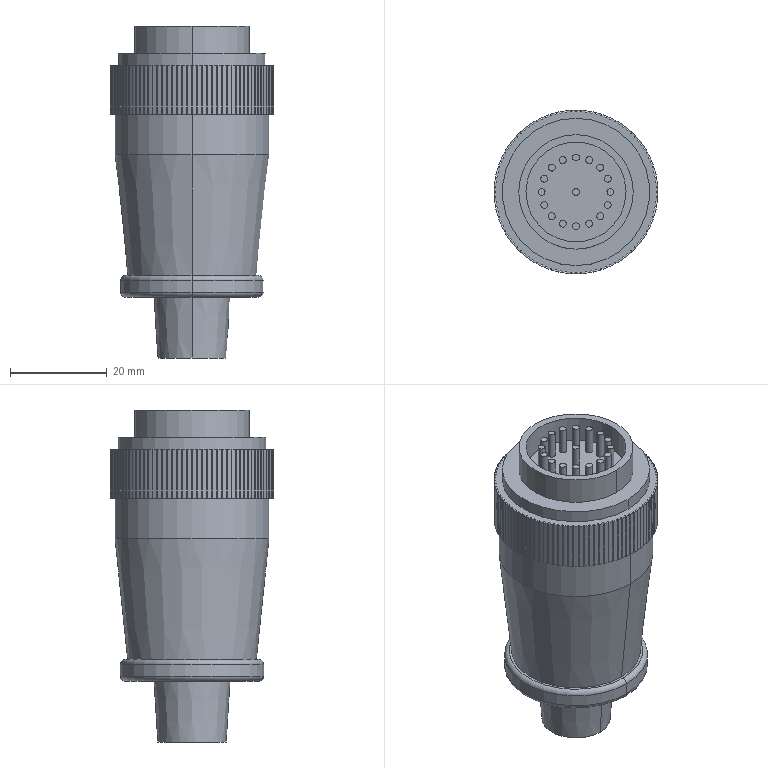Part | STEP file | WS28J26TQ_SW28 | 1 solid | 477 faces | box 33.799 x 33.799 x 68.56 mm | volume 40165 mm3 | plane 325 | cylinder 144 | torus 4 | cone 4 | commonest cylinder face diameters 33.8 x100 1.42 x34 20.66 x2 23.66 x2 29.562 x2 30.42 x2